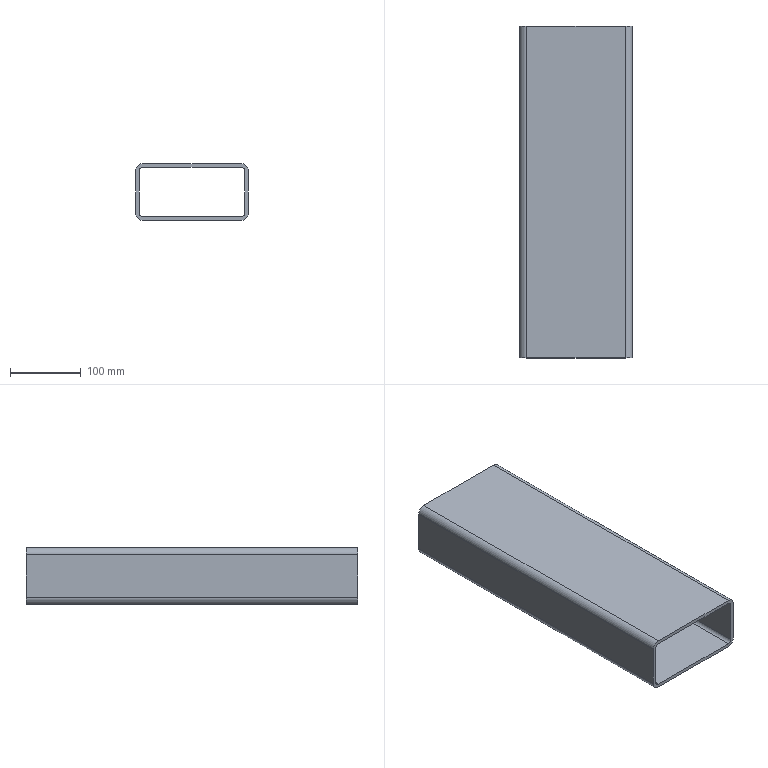Part | SolidWorks | features BaseBody 1 | 1 solid | 26 faces | box 160 x 470 x 80 mm | volume 1049107 mm3 | cylinder 16 | plane 10 | commonest cylinder face diameters 10.2 x8 10 x4 20 x4
STEP:
#1=CARTESIAN_POINT('',(-30.1,174.36,-35.));
#2=VERTEX_POINT('',#1);
#3=CARTESIAN_POINT('',(-19.9,174.36,-35.));
#4=VERTEX_POINT('',#3);
#5=CARTESIAN_POINT('',(-25.,174.36,-35.));
#6=DIRECTION('',(0.,0.,1.));
#7=DIRECTION('',(1.,0.,0.));
#8=AXIS2_PLACEMENT_3D('',#5,#6,#7);
#9=CIRCLE('',#8,5.1);
#10=EDGE_CURVE('',#2,#4,#9,.T.);
#11=ORIENTED_EDGE('',*,*,#10,.T.);
#12=CARTESIAN_POINT('',(-19.9,174.36,-40.));
#13=VERTEX_POINT('',#12);
#14=CARTESIAN_POINT('',(-19.9,174.36,-54.));
#15=DIRECTION('',(0.,0.,-1.));
#16=VECTOR('',#15,1000.);
#17=LINE('',#14,#16);
#18=EDGE_CURVE('',#4,#13,#17,.T.);
#19=ORIENTED_EDGE('',*,*,#18,.T.);
#20=CARTESIAN_POINT('',(-30.1,174.36,-40.));
#21=VERTEX_POINT('',#20);
#22=CARTESIAN_POINT('',(-25.,174.36,-40.));
#23=DIRECTION('',(0.,0.,1.));
#24=DIRECTION('',(1.,0.,0.));
#25=AXIS2_PLACEMENT_3D('',#22,#23,#24);
#26=CIRCLE('',#25,5.1);
#27=EDGE_CURVE('',#21,#13,#26,.T.);
#28=ORIENTED_EDGE('',*,*,#27,.F.);
#29=CARTESIAN_POINT('',(-30.1,174.36,-54.));
#30=DIRECTION('',(0.,0.,-1.));
#31=VECTOR('',#30,1000.);
#32=LINE('',#29,#31);
#33=EDGE_CURVE('',#2,#21,#32,.T.);
#34=ORIENTED_EDGE('',*,*,#33,.F.);
#35=EDGE_LOOP('',(#11,#19,#28,#34));
#36=FACE_OUTER_BOUND('',#35,.T.);
#37=CARTESIAN_POINT('',(-25.,174.36,-54.));
#38=DIRECTION('',(0.,0.,-1.));
#39=DIRECTION('',(-1.,0.,0.));
#40=AXIS2_PLACEMENT_3D('',#37,#38,#39);
#41=CYLINDRICAL_SURFACE('',#40,5.1);
#42=ADVANCED_FACE('',(#36),#41,.F.);
#43=CARTESIAN_POINT('',(29.9,174.36,-35.));
#44=VERTEX_POINT('',#43);
#45=CARTESIAN_POINT('',(40.1,174.36,-35.));
#46=VERTEX_POINT('',#45);
#47=CARTESIAN_POINT('',(35.,174.36,-35.));
#48=DIRECTION('',(0.,0.,1.));
#49=DIRECTION('',(1.,0.,0.));
#50=AXIS2_PLACEMENT_3D('',#47,#48,#49);
#51=CIRCLE('',#50,5.1);
#52=EDGE_CURVE('',#44,#46,#51,.T.);
#53=ORIENTED_EDGE('',*,*,#52,.T.);
#54=CARTESIAN_POINT('',(40.1,174.36,-40.));
#55=VERTEX_POINT('',#54);
#56=CARTESIAN_POINT('',(40.1,174.36,-54.));
#57=DIRECTION('',(0.,0.,-1.));
#58=VECTOR('',#57,1000.);
#59=LINE('',#56,#58);
#60=EDGE_CURVE('',#46,#55,#59,.T.);
#61=ORIENTED_EDGE('',*,*,#60,.T.);
#62=CARTESIAN_POINT('',(29.9,174.36,-40.));
#63=VERTEX_POINT('',#62);
#64=CARTESIAN_POINT('',(35.,174.36,-40.));
#65=DIRECTION('',(0.,0.,1.));
#66=DIRECTION('',(1.,0.,0.));
#67=AXIS2_PLACEMENT_3D('',#64,#65,#66);
#68=CIRCLE('',#67,5.1);
#69=EDGE_CURVE('',#63,#55,#68,.T.);
#70=ORIENTED_EDGE('',*,*,#69,.F.);
#71=CARTESIAN_POINT('',(29.9,174.36,-54.));
#72=DIRECTION('',(0.,0.,-1.));
#73=VECTOR('',#72,1000.);
#74=LINE('',#71,#73);
#75=EDGE_CURVE('',#44,#63,#74,.T.);
#76=ORIENTED_EDGE('',*,*,#75,.F.);
#77=EDGE_LOOP('',(#53,#61,#70,#76));
#78=FACE_OUTER_BOUND('',#77,.T.);
#79=CARTESIAN_POINT('',(35.,174.36,-54.));
#80=DIRECTION('',(0.,0.,-1.));
#81=DIRECTION('',(-1.,0.,0.));
#82=AXIS2_PLACEMENT_3D('',#79,#80,#81);
#83=CYLINDRICAL_SURFACE('',#82,5.1);
#84=ADVANCED_FACE('',(#78),#83,.F.);
#85=CARTESIAN_POINT('',(29.9,54.36,-35.));
#86=VERTEX_POINT('',#85);
#87=CARTESIAN_POINT('',(40.1,54.36,-35.));
#88=VERTEX_POINT('',#87);
#89=CARTESIAN_POINT('',(35.,54.36,-35.));
#90=DIRECTION('',(0.,0.,1.));
#91=DIRECTION('',(1.,0.,0.));
#92=AXIS2_PLACEMENT_3D('',#89,#90,#91);
#93=CIRCLE('',#92,5.1);
#94=EDGE_CURVE('',#86,#88,#93,.T.);
#95=ORIENTED_EDGE('',*,*,#94,.T.);
#96=CARTESIAN_POINT('',(40.1,54.36,-40.));
#97=VERTEX_POINT('',#96);
#98=CARTESIAN_POINT('',(40.1,54.36,-54.));
#99=DIRECTION('',(0.,0.,-1.));
#100=VECTOR('',#99,1000.);
#101=LINE('',#98,#100);
#102=EDGE_CURVE('',#88,#97,#101,.T.);
#103=ORIENTED_EDGE('',*,*,#102,.T.);
#104=CARTESIAN_POINT('',(29.9,54.36,-40.));
#105=VERTEX_POINT('',#104);
#106=CARTESIAN_POINT('',(35.,54.36,-40.));
#107=DIRECTION('',(0.,0.,1.));
#108=DIRECTION('',(1.,0.,0.));
#109=AXIS2_PLACEMENT_3D('',#106,#107,#108);
#110=CIRCLE('',#109,5.1);
#111=EDGE_CURVE('',#105,#97,#110,.T.);
#112=ORIENTED_EDGE('',*,*,#111,.F.);
#113=CARTESIAN_POINT('',(29.9,54.36,-54.));
#114=DIRECTION('',(0.,0.,-1.));
#115=VECTOR('',#114,1000.);
#116=LINE('',#113,#115);
#117=EDGE_CURVE('',#86,#105,#116,.T.);
#118=ORIENTED_EDGE('',*,*,#117,.F.);
#119=EDGE_LOOP('',(#95,#103,#112,#118));
#120=FACE_OUTER_BOUND('',#119,.T.);
#121=CARTESIAN_POINT('',(35.,54.36,-54.));
#122=DIRECTION('',(0.,0.,-1.));
#123=DIRECTION('',(-1.,0.,0.));
#124=AXIS2_PLACEMENT_3D('',#121,#122,#123);
#125=CYLINDRICAL_SURFACE('',#124,5.1);
#126=ADVANCED_FACE('',(#120),#125,.F.);
#127=CARTESIAN_POINT('',(-30.1,54.36,-35.));
#128=VERTEX_POINT('',#127);
#129=CARTESIAN_POINT('',(-19.9,54.36,-35.));
#130=VERTEX_POINT('',#129);
#131=CARTESIAN_POINT('',(-25.,54.36,-35.));
#132=DIRECTION('',(0.,0.,1.));
#133=DIRECTION('',(1.,0.,0.));
#134=AXIS2_PLACEMENT_3D('',#131,#132,#133);
#135=CIRCLE('',#134,5.1);
#136=EDGE_CURVE('',#128,#130,#135,.T.);
#137=ORIENTED_EDGE('',*,*,#136,.T.);
#138=CARTESIAN_POINT('',(-19.9,54.36,-40.));
#139=VERTEX_POINT('',#138);
#140=CARTESIAN_POINT('',(-19.9,54.36,-54.));
#141=DIRECTION('',(0.,0.,-1.));
#142=VECTOR('',#141,1000.);
#143=LINE('',#140,#142);
#144=EDGE_CURVE('',#130,#139,#143,.T.);
#145=ORIENTED_EDGE('',*,*,#144,.T.);
#146=CARTESIAN_POINT('',(-30.1,54.36,-40.));
#147=VERTEX_POINT('',#146);
#148=CARTESIAN_POINT('',(-25.,54.36,-40.));
#149=DIRECTION('',(0.,0.,1.));
#150=DIRECTION('',(1.,0.,0.));
#151=AXIS2_PLACEMENT_3D('',#148,#149,#150);
#152=CIRCLE('',#151,5.1);
#153=EDGE_CURVE('',#147,#139,#152,.T.);
#154=ORIENTED_EDGE('',*,*,#153,.F.);
#155=CARTESIAN_POINT('',(-30.1,54.36,-54.));
#156=DIRECTION('',(0.,0.,-1.));
#157=VECTOR('',#156,1000.);
#158=LINE('',#155,#157);
#159=EDGE_CURVE('',#128,#147,#158,.T.);
#160=ORIENTED_EDGE('',*,*,#159,.F.);
#161=EDGE_LOOP('',(#137,#145,#154,#160));
#162=FACE_OUTER_BOUND('',#161,.T.);
#163=CARTESIAN_POINT('',(-25.,54.36,-54.));
#164=DIRECTION('',(0.,0.,-1.));
#165=DIRECTION('',(-1.,0.,0.));
#166=AXIS2_PLACEMENT_3D('',#163,#164,#165);
#167=CYLINDRICAL_SURFACE('',#166,5.1);
#168=ADVANCED_FACE('',(#162),#167,.F.);
#169=CARTESIAN_POINT('',(-70.,235.,40.));
#170=VERTEX_POINT('',#169);
#171=CARTESIAN_POINT('',(-80.,235.,30.));
#172=VERTEX_POINT('',#171);
#173=CARTESIAN_POINT('',(-70.,235.,30.));
#174=DIRECTION('',(0.,-1.,0.));
#175=DIRECTION('',(1.,0.,0.));
#176=AXIS2_PLACEMENT_3D('',#173,#174,#175);
#177=CIRCLE('',#176,10.);
#178=EDGE_CURVE('',#170,#172,#177,.T.);
#179=ORIENTED_EDGE('',*,*,#178,.T.);
#180=CARTESIAN_POINT('',(-80.,-235.,30.));
#181=VERTEX_POINT('',#180);
#182=CARTESIAN_POINT('',(-80.,-235.,30.));
#183=DIRECTION('',(0.,1.,0.));
#184=VECTOR('',#183,1000.);
#185=LINE('',#182,#184);
#186=EDGE_CURVE('',#181,#172,#185,.T.);
#187=ORIENTED_EDGE('',*,*,#186,.F.);
#188=CARTESIAN_POINT('',(-70.,-235.,40.));
#189=VERTEX_POINT('',#188);
#190=CARTESIAN_POINT('',(-70.,-235.,30.));
#191=DIRECTION('',(0.,-1.,0.));
#192=DIRECTION('',(1.,0.,0.));
#193=AXIS2_PLACEMENT_3D('',#190,#191,#192);
#194=CIRCLE('',#193,10.);
#195=EDGE_CURVE('',#189,#181,#194,.T.);
#196=ORIENTED_EDGE('',*,*,#195,.F.);
#197=CARTESIAN_POINT('',(-70.,-235.,40.));
#198=DIRECTION('',(0.,1.,0.));
#199=VECTOR('',#198,1000.);
#200=LINE('',#197,#199);
#201=EDGE_CURVE('',#189,#170,#200,.T.);
#202=ORIENTED_EDGE('',*,*,#201,.T.);
#203=EDGE_LOOP('',(#179,#187,#196,#202));
#204=FACE_OUTER_BOUND('',#203,.T.);
#205=CARTESIAN_POINT('',(-70.,-235.,30.));
#206=DIRECTION('',(0.,1.,0.));
#207=DIRECTION('',(-1.,0.,0.));
#208=AXIS2_PLACEMENT_3D('',#205,#206,#207);
#209=CYLINDRICAL_SURFACE('',#208,10.);
#210=ADVANCED_FACE('',(#204),#209,.T.);
#211=CARTESIAN_POINT('',(-80.,235.,-30.));
#212=VERTEX_POINT('',#211);
#213=CARTESIAN_POINT('',(-80.,235.,30.));
#214=DIRECTION('',(0.,0.,-1.));
#215=VECTOR('',#214,1000.);
#216=LINE('',#213,#215);
#217=EDGE_CURVE('',#172,#212,#216,.T.);
#218=ORIENTED_EDGE('',*,*,#217,.T.);
#219=CARTESIAN_POINT('',(-80.,-235.,-30.));
#220=VERTEX_POINT('',#219);
#221=CARTESIAN_POINT('',(-80.,-235.,-30.));
#222=DIRECTION('',(0.,1.,0.));
#223=VECTOR('',#222,1000.);
#224=LINE('',#221,#223);
#225=EDGE_CURVE('',#220,#212,#224,.T.);
#226=ORIENTED_EDGE('',*,*,#225,.F.);
#227=CARTESIAN_POINT('',(-80.,-235.,30.));
#228=DIRECTION('',(0.,0.,-1.));
#229=VECTOR('',#228,1000.);
#230=LINE('',#227,#229);
#231=EDGE_CURVE('',#181,#220,#230,.T.);
#232=ORIENTED_EDGE('',*,*,#231,.F.);
#233=ORIENTED_EDGE('',*,*,#186,.T.);
#234=EDGE_LOOP('',(#218,#226,#232,#233));
#235=FACE_OUTER_BOUND('',#234,.T.);
#236=CARTESIAN_POINT('',(-80.,-235.,30.));
#237=DIRECTION('',(1.,0.,0.));
#238=DIRECTION('',(0.,0.,-1.));
#239=AXIS2_PLACEMENT_3D('',#236,#237,#238);
#240=PLANE('',#239);
#241=ADVANCED_FACE('',(#235),#240,.F.);
#242=CARTESIAN_POINT('',(-70.,235.,-40.));
#243=VERTEX_POINT('',#242);
#244=CARTESIAN_POINT('',(-70.,235.,-30.));
#245=DIRECTION('',(0.,-1.,0.));
#246=DIRECTION('',(1.,0.,0.));
#247=AXIS2_PLACEMENT_3D('',#244,#245,#246);
#248=CIRCLE('',#247,10.);
#249=EDGE_CURVE('',#212,#243,#248,.T.);
#250=ORIENTED_EDGE('',*,*,#249,.T.);
#251=CARTESIAN_POINT('',(-70.,-235.,-40.));
#252=VERTEX_POINT('',#251);
#253=CARTESIAN_POINT('',(-70.,-235.,-40.));
#254=DIRECTION('',(0.,1.,0.));
#255=VECTOR('',#254,1000.);
#256=LINE('',#253,#255);
#257=EDGE_CURVE('',#252,#243,#256,.T.);
#258=ORIENTED_EDGE('',*,*,#257,.F.);
#259=CARTESIAN_POINT('',(-70.,-235.,-30.));
#260=DIRECTION('',(0.,-1.,0.));
#261=DIRECTION('',(1.,0.,0.));
#262=AXIS2_PLACEMENT_3D('',#259,#260,#261);
#263=CIRCLE('',#262,10.);
#264=EDGE_CURVE('',#220,#252,#263,.T.);
#265=ORIENTED_EDGE('',*,*,#264,.F.);
#266=ORIENTED_EDGE('',*,*,#225,.T.);
#267=EDGE_LOOP('',(#250,#258,#265,#266));
#268=FACE_OUTER_BOUND('',#267,.T.);
#269=CARTESIAN_POINT('',(-70.,-235.,-30.));
#270=DIRECTION('',(0.,1.,0.));
#271=DIRECTION('',(-1.,0.,0.));
#272=AXIS2_PLACEMENT_3D('',#269,#270,#271);
#273=CYLINDRICAL_SURFACE('',#272,10.);
#274=ADVANCED_FACE('',(#268),#273,.T.);
#275=ORIENTED_EDGE('',*,*,#27,.T.);
#276=CARTESIAN_POINT('',(-25.,174.36,-40.));
#277=DIRECTION('',(0.,0.,1.));
#278=DIRECTION('',(1.,0.,0.));
#279=AXIS2_PLACEMENT_3D('',#276,#277,#278);
#280=CIRCLE('',#279,5.1);
#281=EDGE_CURVE('',#13,#21,#280,.T.);
#282=ORIENTED_EDGE('',*,*,#281,.T.);
#283=EDGE_LOOP('',(#275,#282));
#284=FACE_BOUND('',#283,.T.);
#285=ORIENTED_EDGE('',*,*,#69,.T.);
#286=CARTESIAN_POINT('',(35.,174.36,-40.));
#287=DIRECTION('',(0.,0.,1.));
#288=DIRECTION('',(1.,0.,0.));
#289=AXIS2_PLACEMENT_3D('',#286,#287,#288);
#290=CIRCLE('',#289,5.1);
#291=EDGE_CURVE('',#55,#63,#290,.T.);
#292=ORIENTED_EDGE('',*,*,#291,.T.);
#293=EDGE_LOOP('',(#285,#292));
#294=FACE_BOUND('',#293,.T.);
#295=ORIENTED_EDGE('',*,*,#111,.T.);
#296=CARTESIAN_POINT('',(35.,54.36,-40.));
#297=DIRECTION('',(0.,0.,1.));
#298=DIRECTION('',(1.,0.,0.));
#299=AXIS2_PLACEMENT_3D('',#296,#297,#298);
#300=CIRCLE('',#299,5.1);
#301=EDGE_CURVE('',#97,#105,#300,.T.);
#302=ORIENTED_EDGE('',*,*,#301,.T.);
#303=EDGE_LOOP('',(#295,#302));
#304=FACE_BOUND('',#303,.T.);
#305=ORIENTED_EDGE('',*,*,#153,.T.);
#306=CARTESIAN_POINT('',(-25.,54.36,-40.));
#307=DIRECTION('',(0.,0.,1.));
#308=DIRECTION('',(1.,0.,0.));
#309=AXIS2_PLACEMENT_3D('',#306,#307,#308);
#310=CIRCLE('',#309,5.1);
#311=EDGE_CURVE('',#139,#147,#310,.T.);
#312=ORIENTED_EDGE('',*,*,#311,.T.);
#313=EDGE_LOOP('',(#305,#312));
#314=FACE_BOUND('',#313,.T.);
#315=CARTESIAN_POINT('',(70.,235.,-40.));
#316=VERTEX_POINT('',#315);
#317=CARTESIAN_POINT('',(70.,235.,-40.));
#318=DIRECTION('',(1.,0.,0.));
#319=VECTOR('',#318,1000.);
#320=LINE('',#317,#319);
#321=EDGE_CURVE('',#243,#316,#320,.T.);
#322=ORIENTED_EDGE('',*,*,#321,.T.);
#323=CARTESIAN_POINT('',(70.,-235.,-40.));
#324=VERTEX_POINT('',#323);
#325=CARTESIAN_POINT('',(70.,-235.,-40.));
#326=DIRECTION('',(0.,1.,0.));
#327=VECTOR('',#326,1000.);
#328=LINE('',#325,#327);
#329=EDGE_CURVE('',#324,#316,#328,.T.);
#330=ORIENTED_EDGE('',*,*,#329,.F.);
#331=CARTESIAN_POINT('',(70.,-235.,-40.));
#332=DIRECTION('',(1.,0.,0.));
#333=VECTOR('',#332,1000.);
#334=LINE('',#331,#333);
#335=EDGE_CURVE('',#252,#324,#334,.T.);
#336=ORIENTED_EDGE('',*,*,#335,.F.);
#337=ORIENTED_EDGE('',*,*,#257,.T.);
#338=EDGE_LOOP('',(#322,#330,#336,#337));
#339=FACE_OUTER_BOUND('',#338,.T.);
#340=CARTESIAN_POINT('',(70.,-235.,-40.));
#341=DIRECTION('',(0.,0.,1.));
#342=DIRECTION('',(1.,0.,0.));
#343=AXIS2_PLACEMENT_3D('',#340,#341,#342);
#344=PLANE('',#343);
#345=ADVANCED_FACE('',(#284,#294,#304,#314,#339),#344,.F.);
#346=CARTESIAN_POINT('',(80.,235.,-30.));
#347=VERTEX_POINT('',#346);
#348=CARTESIAN_POINT('',(70.,235.,-30.));
#349=DIRECTION('',(0.,-1.,0.));
#350=DIRECTION('',(1.,0.,0.));
#351=AXIS2_PLACEMENT_3D('',#348,#349,#350);
#352=CIRCLE('',#351,10.);
#353=EDGE_CURVE('',#316,#347,#352,.T.);
#354=ORIENTED_EDGE('',*,*,#353,.T.);
#355=CARTESIAN_POINT('',(80.,-235.,-30.));
#356=VERTEX_POINT('',#355);
#357=CARTESIAN_POINT('',(80.,-235.,-30.));
#358=DIRECTION('',(0.,1.,0.));
#359=VECTOR('',#358,1000.);
#360=LINE('',#357,#359);
#361=EDGE_CURVE('',#356,#347,#360,.T.);
#362=ORIENTED_EDGE('',*,*,#361,.F.);
#363=CARTESIAN_POINT('',(70.,-235.,-30.));
#364=DIRECTION('',(0.,-1.,0.));
#365=DIRECTION('',(1.,0.,0.));
#366=AXIS2_PLACEMENT_3D('',#363,#364,#365);
#367=CIRCLE('',#366,10.);
#368=EDGE_CURVE('',#324,#356,#367,.T.);
#369=ORIENTED_EDGE('',*,*,#368,.F.);
#370=ORIENTED_EDGE('',*,*,#329,.T.);
#371=EDGE_LOOP('',(#354,#362,#369,#370));
#372=FACE_OUTER_BOUND('',#371,.T.);
#373=CARTESIAN_POINT('',(70.,-235.,-30.));
#374=DIRECTION('',(0.,1.,0.));
#375=DIRECTION('',(-1.,0.,0.));
#376=AXIS2_PLACEMENT_3D('',#373,#374,#375);
#377=CYLINDRICAL_SURFACE('',#376,10.);
#378=ADVANCED_FACE('',(#372),#377,.T.);
#379=CARTESIAN_POINT('',(80.,235.,30.));
#380=VERTEX_POINT('',#379);
#381=CARTESIAN_POINT('',(80.,235.,-30.));
#382=DIRECTION('',(0.,0.,1.));
#383=VECTOR('',#382,1000.);
#384=LINE('',#381,#383);
#385=EDGE_CURVE('',#347,#380,#384,.T.);
#386=ORIENTED_EDGE('',*,*,#385,.T.);
#387=CARTESIAN_POINT('',(80.,-235.,30.));
#388=VERTEX_POINT('',#387);
#389=CARTESIAN_POINT('',(80.,-235.,30.));
#390=DIRECTION('',(0.,1.,0.));
#391=VECTOR('',#390,1000.);
#392=LINE('',#389,#391);
#393=EDGE_CURVE('',#388,#380,#392,.T.);
#394=ORIENTED_EDGE('',*,*,#393,.F.);
#395=CARTESIAN_POINT('',(80.,-235.,-30.));
#396=DIRECTION('',(0.,0.,1.));
#397=VECTOR('',#396,1000.);
#398=LINE('',#395,#397);
#399=EDGE_CURVE('',#356,#388,#398,.T.);
#400=ORIENTED_EDGE('',*,*,#399,.F.);
#401=ORIENTED_EDGE('',*,*,#361,.T.);
#402=EDGE_LOOP('',(#386,#394,#400,#401));
#403=FACE_OUTER_BOUND('',#402,.T.);
#404=CARTESIAN_POINT('',(80.,-235.,-30.));
#405=DIRECTION('',(-1.,0.,0.));
#406=DIRECTION('',(0.,0.,1.));
#407=AXIS2_PLACEMENT_3D('',#404,#405,#406);
#408=PLANE('',#407);
#409=ADVANCED_FACE('',(#403),#408,.F.);
#410=CARTESIAN_POINT('',(70.,235.,40.));
#411=VERTEX_POINT('',#410);
#412=CARTESIAN_POINT('',(70.,235.,30.));
#413=DIRECTION('',(0.,-1.,0.));
#414=DIRECTION('',(1.,0.,0.));
#415=AXIS2_PLACEMENT_3D('',#412,#413,#414);
#416=CIRCLE('',#415,10.);
#417=EDGE_CURVE('',#380,#411,#416,.T.);
#418=ORIENTED_EDGE('',*,*,#417,.T.);
#419=CARTESIAN_POINT('',(70.,-235.,40.));
#420=VERTEX_POINT('',#419);
#421=CARTESIAN_POINT('',(70.,-235.,40.));
#422=DIRECTION('',(0.,1.,0.));
#423=VECTOR('',#422,1000.);
#424=LINE('',#421,#423);
#425=EDGE_CURVE('',#420,#411,#424,.T.);
#426=ORIENTED_EDGE('',*,*,#425,.F.);
#427=CARTESIAN_POINT('',(70.,-235.,30.));
#428=DIRECTION('',(0.,-1.,0.));
#429=DIRECTION('',(1.,0.,0.));
#430=AXIS2_PLACEMENT_3D('',#427,#428,#429);
#431=CIRCLE('',#430,10.);
#432=EDGE_CURVE('',#388,#420,#431,.T.);
#433=ORIENTED_EDGE('',*,*,#432,.F.);
#434=ORIENTED_EDGE('',*,*,#393,.T.);
#435=EDGE_LOOP('',(#418,#426,#433,#434));
#436=FACE_OUTER_BOUND('',#435,.T.);
#437=CARTESIAN_POINT('',(70.,-235.,30.));
#438=DIRECTION('',(0.,1.,0.));
#439=DIRECTION('',(-1.,0.,0.));
#440=AXIS2_PLACEMENT_3D('',#437,#438,#439);
#441=CYLINDRICAL_SURFACE('',#440,10.);
#442=ADVANCED_FACE('',(#436),#441,.T.);
#443=CARTESIAN_POINT('',(-75.,235.,-30.));
#444=VERTEX_POINT('',#443);
#445=CARTESIAN_POINT('',(-70.,235.,-35.));
#446=VERTEX_POINT('',#445);
#447=CARTESIAN_POINT('',(-70.,235.,-30.));
#448=DIRECTION('',(0.,-1.,0.));
#449=DIRECTION('',(1.,0.,0.));
#450=AXIS2_PLACEMENT_3D('',#447,#448,#449);
#451=CIRCLE('',#450,5.);
#452=EDGE_CURVE('',#444,#446,#451,.T.);
#453=ORIENTED_EDGE('',*,*,#452,.F.);
#454=CARTESIAN_POINT('',(-75.,-235.,-30.));
#455=VERTEX_POINT('',#454);
#456=CARTESIAN_POINT('',(-75.,-235.,-30.));
#457=DIRECTION('',(0.,1.,0.));
#458=VECTOR('',#457,1000.);
#459=LINE('',#456,#458);
#460=EDGE_CURVE('',#455,#444,#459,.T.);
#461=ORIENTED_EDGE('',*,*,#460,.F.);
#462=CARTESIAN_POINT('',(-70.,-235.,-35.));
#463=VERTEX_POINT('',#462);
#464=CARTESIAN_POINT('',(-70.,-235.,-30.));
#465=DIRECTION('',(0.,-1.,0.));
#466=DIRECTION('',(1.,0.,0.));
#467=AXIS2_PLACEMENT_3D('',#464,#465,#466);
#468=CIRCLE('',#467,5.);
#469=EDGE_CURVE('',#455,#463,#468,.T.);
#470=ORIENTED_EDGE('',*,*,#469,.T.);
#471=CARTESIAN_POINT('',(-70.,-235.,-35.));
#472=DIRECTION('',(0.,1.,0.));
#473=VECTOR('',#472,1000.);
#474=LINE('',#471,#473);
#475=EDGE_CURVE('',#463,#446,#474,.T.);
#476=ORIENTED_EDGE('',*,*,#475,.T.);
#477=EDGE_LOOP('',(#453,#461,#470,#476));
#478=FACE_OUTER_BOUND('',#477,.T.);
#479=CARTESIAN_POINT('',(-70.,-235.,-30.));
#480=DIRECTION('',(0.,1.,0.));
#481=DIRECTION('',(-1.,0.,0.));
#482=AXIS2_PLACEMENT_3D('',#479,#480,#481);
#483=CYLINDRICAL_SURFACE('',#482,5.);
#484=ADVANCED_FACE('',(#478),#483,.F.);
#485=CARTESIAN_POINT('',(-75.,235.,30.));
#486=VERTEX_POINT('',#485);
#487=CARTESIAN_POINT('',(-75.,235.,30.));
#488=DIRECTION('',(0.,0.,-1.));
#489=VECTOR('',#488,1000.);
#490=LINE('',#487,#489);
#491=EDGE_CURVE('',#486,#444,#490,.T.);
#492=ORIENTED_EDGE('',*,*,#491,.F.);
#493=CARTESIAN_POINT('',(-75.,-235.,30.));
#494=VERTEX_POINT('',#493);
#495=CARTESIAN_POINT('',(-75.,-235.,30.));
#496=DIRECTION('',(0.,1.,0.));
#497=VECTOR('',#496,1000.);
#498=LINE('',#495,#497);
#499=EDGE_CURVE('',#494,#486,#498,.T.);
#500=ORIENTED_EDGE('',*,*,#499,.F.);
#501=CARTESIAN_POINT('',(-75.,-235.,30.));
#502=DIRECTION('',(0.,0.,-1.));
#503=VECTOR('',#502,1000.);
#504=LINE('',#501,#503);
#505=EDGE_CURVE('',#494,#455,#504,.T.);
#506=ORIENTED_EDGE('',*,*,#505,.T.);
#507=ORIENTED_EDGE('',*,*,#460,.T.);
#508=EDGE_LOOP('',(#492,#500,#506,#507));
#509=FACE_OUTER_BOUND('',#508,.T.);
#510=CARTESIAN_POINT('',(-75.,-235.,30.));
#511=DIRECTION('',(1.,0.,0.));
#512=DIRECTION('',(0.,0.,-1.));
#513=AXIS2_PLACEMENT_3D('',#510,#511,#512);
#514=PLANE('',#513);
#515=ADVANCED_FACE('',(#509),#514,.T.);
#516=CARTESIAN_POINT('',(-70.,235.,35.));
#517=VERTEX_POINT('',#516);
#518=CARTESIAN_POINT('',(-70.,235.,30.));
#519=DIRECTION('',(0.,-1.,0.));
#520=DIRECTION('',(1.,0.,0.));
#521=AXIS2_PLACEMENT_3D('',#518,#519,#520);
#522=CIRCLE('',#521,5.);
#523=EDGE_CURVE('',#517,#486,#522,.T.);
#524=ORIENTED_EDGE('',*,*,#523,.F.);
#525=CARTESIAN_POINT('',(-70.,-235.,35.));
#526=VERTEX_POINT('',#525);
#527=CARTESIAN_POINT('',(-70.,-235.,35.));
#528=DIRECTION('',(0.,1.,0.));
#529=VECTOR('',#528,1000.);
#530=LINE('',#527,#529);
#531=EDGE_CURVE('',#526,#517,#530,.T.);
#532=ORIENTED_EDGE('',*,*,#531,.F.);
#533=CARTESIAN_POINT('',(-70.,-235.,30.));
#534=DIRECTION('',(0.,-1.,0.));
#535=DIRECTION('',(1.,0.,0.));
#536=AXIS2_PLACEMENT_3D('',#533,#534,#535);
#537=CIRCLE('',#536,5.);
#538=EDGE_CURVE('',#526,#494,#537,.T.);
#539=ORIENTED_EDGE('',*,*,#538,.T.);
#540=ORIENTED_EDGE('',*,*,#499,.T.);
#541=EDGE_LOOP('',(#524,#532,#539,#540));
#542=FACE_OUTER_BOUND('',#541,.T.);
#543=CARTESIAN_POINT('',(-70.,-235.,30.));
#544=DIRECTION('',(0.,1.,0.));
#545=DIRECTION('',(-1.,0.,0.));
#546=AXIS2_PLACEMENT_3D('',#543,#544,#545);
#547=CYLINDRICAL_SURFACE('',#546,5.);
#548=ADVANCED_FACE('',(#542),#547,.F.);
#549=CARTESIAN_POINT('',(70.,235.,35.));
#550=VERTEX_POINT('',#549);
#551=CARTESIAN_POINT('',(-70.,235.,35.));
#552=DIRECTION('',(-1.,0.,0.));
#553=VECTOR('',#552,1000.);
#554=LINE('',#551,#553);
#555=EDGE_CURVE('',#550,#517,#554,.T.);
#556=ORIENTED_EDGE('',*,*,#555,.F.);
#557=CARTESIAN_POINT('',(70.,-235.,35.));
#558=VERTEX_POINT('',#557);
#559=CARTESIAN_POINT('',(70.,-235.,35.));
#560=DIRECTION('',(0.,1.,0.));
#561=VECTOR('',#560,1000.);
#562=LINE('',#559,#561);
#563=EDGE_CURVE('',#558,#550,#562,.T.);
#564=ORIENTED_EDGE('',*,*,#563,.F.);
#565=CARTESIAN_POINT('',(-70.,-235.,35.));
#566=DIRECTION('',(-1.,0.,0.));
#567=VECTOR('',#566,1000.);
#568=LINE('',#565,#567);
#569=EDGE_CURVE('',#558,#526,#568,.T.);
#570=ORIENTED_EDGE('',*,*,#569,.T.);
#571=ORIENTED_EDGE('',*,*,#531,.T.);
#572=EDGE_LOOP('',(#556,#564,#570,#571));
#573=FACE_OUTER_BOUND('',#572,.T.);
#574=CARTESIAN_POINT('',(-70.,-235.,35.));
#575=DIRECTION('',(0.,0.,-1.));
#576=DIRECTION('',(-1.,0.,0.));
#577=AXIS2_PLACEMENT_3D('',#574,#575,#576);
#578=PLANE('',#577);
#579=ADVANCED_FACE('',(#573),#578,.T.);
#580=CARTESIAN_POINT('',(75.,235.,30.));
#581=VERTEX_POINT('',#580);
#582=CARTESIAN_POINT('',(70.,235.,30.));
#583=DIRECTION('',(0.,-1.,0.));
#584=DIRECTION('',(1.,0.,0.));
#585=AXIS2_PLACEMENT_3D('',#582,#583,#584);
#586=CIRCLE('',#585,5.);
#587=EDGE_CURVE('',#581,#550,#586,.T.);
#588=ORIENTED_EDGE('',*,*,#587,.F.);
#589=CARTESIAN_POINT('',(75.,-235.,30.));
#590=VERTEX_POINT('',#589);
#591=CARTESIAN_POINT('',(75.,-235.,30.));
#592=DIRECTION('',(0.,1.,0.));
#593=VECTOR('',#592,1000.);
#594=LINE('',#591,#593);
#595=EDGE_CURVE('',#590,#581,#594,.T.);
#596=ORIENTED_EDGE('',*,*,#595,.F.);
#597=CARTESIAN_POINT('',(70.,-235.,30.));
#598=DIRECTION('',(0.,-1.,0.));
#599=DIRECTION('',(1.,0.,0.));
#600=AXIS2_PLACEMENT_3D('',#597,#598,#599);
#601=CIRCLE('',#600,5.);
#602=EDGE_CURVE('',#590,#558,#601,.T.);
#603=ORIENTED_EDGE('',*,*,#602,.T.);
#604=ORIENTED_EDGE('',*,*,#563,.T.);
#605=EDGE_LOOP('',(#588,#596,#603,#604));
#606=FACE_OUTER_BOUND('',#605,.T.);
#607=CARTESIAN_POINT('',(70.,-235.,30.));
#608=DIRECTION('',(0.,1.,0.));
#609=DIRECTION('',(-1.,0.,0.));
#610=AXIS2_PLACEMENT_3D('',#607,#608,#609);
#611=CYLINDRICAL_SURFACE('',#610,5.);
#612=ADVANCED_FACE('',(#606),#611,.F.);
#613=CARTESIAN_POINT('',(75.,235.,-30.));
#614=VERTEX_POINT('',#613);
#615=CARTESIAN_POINT('',(75.,235.,-30.));
#616=DIRECTION('',(0.,0.,1.));
#617=VECTOR('',#616,1000.);
#618=LINE('',#615,#617);
#619=EDGE_CURVE('',#614,#581,#618,.T.);
#620=ORIENTED_EDGE('',*,*,#619,.F.);
#621=CARTESIAN_POINT('',(75.,-235.,-30.));
#622=VERTEX_POINT('',#621);
#623=CARTESIAN_POINT('',(75.,-235.,-30.));
#624=DIRECTION('',(0.,1.,0.));
#625=VECTOR('',#624,1000.);
#626=LINE('',#623,#625);
#627=EDGE_CURVE('',#622,#614,#626,.T.);
#628=ORIENTED_EDGE('',*,*,#627,.F.);
#629=CARTESIAN_POINT('',(75.,-235.,-30.));
#630=DIRECTION('',(0.,0.,1.));
#631=VECTOR('',#630,1000.);
#632=LINE('',#629,#631);
#633=EDGE_CURVE('',#622,#590,#632,.T.);
#634=ORIENTED_EDGE('',*,*,#633,.T.);
#635=ORIENTED_EDGE('',*,*,#595,.T.);
#636=EDGE_LOOP('',(#620,#628,#634,#635));
#637=FACE_OUTER_BOUND('',#636,.T.);
#638=CARTESIAN_POINT('',(75.,-235.,-30.));
#639=DIRECTION('',(-1.,0.,0.));
#640=DIRECTION('',(0.,0.,1.));
#641=AXIS2_PLACEMENT_3D('',#638,#639,#640);
#642=PLANE('',#641);
#643=ADVANCED_FACE('',(#637),#642,.T.);
#644=CARTESIAN_POINT('',(70.,235.,-35.));
#645=VERTEX_POINT('',#644);
#646=CARTESIAN_POINT('',(70.,235.,-30.));
#647=DIRECTION('',(0.,-1.,0.));
#648=DIRECTION('',(1.,0.,0.));
#649=AXIS2_PLACEMENT_3D('',#646,#647,#648);
#650=CIRCLE('',#649,5.);
#651=EDGE_CURVE('',#645,#614,#650,.T.);
#652=ORIENTED_EDGE('',*,*,#651,.F.);
#653=CARTESIAN_POINT('',(70.,-235.,-35.));
#654=VERTEX_POINT('',#653);
#655=CARTESIAN_POINT('',(70.,-235.,-35.));
#656=DIRECTION('',(0.,1.,0.));
#657=VECTOR('',#656,1000.);
#658=LINE('',#655,#657);
#659=EDGE_CURVE('',#654,#645,#658,.T.);
#660=ORIENTED_EDGE('',*,*,#659,.F.);
#661=CARTESIAN_POINT('',(70.,-235.,-30.));
#662=DIRECTION('',(0.,-1.,0.));
#663=DIRECTION('',(1.,0.,0.));
#664=AXIS2_PLACEMENT_3D('',#661,#662,#663);
#665=CIRCLE('',#664,5.);
#666=EDGE_CURVE('',#654,#622,#665,.T.);
#667=ORIENTED_EDGE('',*,*,#666,.T.);
#668=ORIENTED_EDGE('',*,*,#627,.T.);
#669=EDGE_LOOP('',(#652,#660,#667,#668));
#670=FACE_OUTER_BOUND('',#669,.T.);
#671=CARTESIAN_POINT('',(70.,-235.,-30.));
#672=DIRECTION('',(0.,1.,0.));
#673=DIRECTION('',(-1.,0.,0.));
#674=AXIS2_PLACEMENT_3D('',#671,#672,#673);
#675=CYLINDRICAL_SURFACE('',#674,5.);
#676=ADVANCED_FACE('',(#670),#675,.F.);
#677=ORIENTED_EDGE('',*,*,#10,.F.);
#678=CARTESIAN_POINT('',(-25.,174.36,-35.));
#679=DIRECTION('',(0.,0.,1.));
#680=DIRECTION('',(1.,0.,0.));
#681=AXIS2_PLACEMENT_3D('',#678,#679,#680);
#682=CIRCLE('',#681,5.1);
#683=EDGE_CURVE('',#4,#2,#682,.T.);
#684=ORIENTED_EDGE('',*,*,#683,.F.);
#685=EDGE_LOOP('',(#677,#684));
#686=FACE_BOUND('',#685,.T.);
#687=ORIENTED_EDGE('',*,*,#52,.F.);
#688=CARTESIAN_POINT('',(35.,174.36,-35.));
#689=DIRECTION('',(0.,0.,1.));
#690=DIRECTION('',(1.,0.,0.));
#691=AXIS2_PLACEMENT_3D('',#688,#689,#690);
#692=CIRCLE('',#691,5.1);
#693=EDGE_CURVE('',#46,#44,#692,.T.);
#694=ORIENTED_EDGE('',*,*,#693,.F.);
#695=EDGE_LOOP('',(#687,#694));
#696=FACE_BOUND('',#695,.T.);
#697=ORIENTED_EDGE('',*,*,#94,.F.);
#698=CARTESIAN_POINT('',(35.,54.36,-35.));
#699=DIRECTION('',(0.,0.,1.));
#700=DIRECTION('',(1.,0.,0.));
#701=AXIS2_PLACEMENT_3D('',#698,#699,#700);
#702=CIRCLE('',#701,5.1);
#703=EDGE_CURVE('',#88,#86,#702,.T.);
#704=ORIENTED_EDGE('',*,*,#703,.F.);
#705=EDGE_LOOP('',(#697,#704));
#706=FACE_BOUND('',#705,.T.);
#707=ORIENTED_EDGE('',*,*,#136,.F.);
#708=CARTESIAN_POINT('',(-25.,54.36,-35.));
#709=DIRECTION('',(0.,0.,1.));
#710=DIRECTION('',(1.,0.,0.));
#711=AXIS2_PLACEMENT_3D('',#708,#709,#710);
#712=CIRCLE('',#711,5.1);
#713=EDGE_CURVE('',#130,#128,#712,.T.);
#714=ORIENTED_EDGE('',*,*,#713,.F.);
#715=EDGE_LOOP('',(#707,#714));
#716=FACE_BOUND('',#715,.T.);
#717=CARTESIAN_POINT('',(70.,235.,-35.));
#718=DIRECTION('',(1.,0.,0.));
#719=VECTOR('',#718,1000.);
#720=LINE('',#717,#719);
#721=EDGE_CURVE('',#446,#645,#720,.T.);
#722=ORIENTED_EDGE('',*,*,#721,.F.);
#723=ORIENTED_EDGE('',*,*,#475,.F.);
#724=CARTESIAN_POINT('',(70.,-235.,-35.));
#725=DIRECTION('',(1.,0.,0.));
#726=VECTOR('',#725,1000.);
#727=LINE('',#724,#726);
#728=EDGE_CURVE('',#463,#654,#727,.T.);
#729=ORIENTED_EDGE('',*,*,#728,.T.);
#730=ORIENTED_EDGE('',*,*,#659,.T.);
#731=EDGE_LOOP('',(#722,#723,#729,#730));
#732=FACE_OUTER_BOUND('',#731,.T.);
#733=CARTESIAN_POINT('',(70.,-235.,-35.));
#734=DIRECTION('',(0.,0.,1.));
#735=DIRECTION('',(1.,0.,0.));
#736=AXIS2_PLACEMENT_3D('',#733,#734,#735);
#737=PLANE('',#736);
#738=ADVANCED_FACE('',(#686,#696,#706,#716,#732),#737,.T.);
#739=CARTESIAN_POINT('',(-70.,235.,40.));
#740=DIRECTION('',(-1.,0.,0.));
#741=VECTOR('',#740,1000.);
#742=LINE('',#739,#741);
#743=EDGE_CURVE('',#411,#170,#742,.T.);
#744=ORIENTED_EDGE('',*,*,#743,.T.);
#745=ORIENTED_EDGE('',*,*,#201,.F.);
#746=CARTESIAN_POINT('',(-70.,-235.,40.));
#747=DIRECTION('',(-1.,0.,0.));
#748=VECTOR('',#747,1000.);
#749=LINE('',#746,#748);
#750=EDGE_CURVE('',#420,#189,#749,.T.);
#751=ORIENTED_EDGE('',*,*,#750,.F.);
#752=ORIENTED_EDGE('',*,*,#425,.T.);
#753=EDGE_LOOP('',(#744,#745,#751,#752));
#754=FACE_OUTER_BOUND('',#753,.T.);
#755=CARTESIAN_POINT('',(-70.,-235.,40.));
#756=DIRECTION('',(0.,0.,-1.));
#757=DIRECTION('',(-1.,0.,0.));
#758=AXIS2_PLACEMENT_3D('',#755,#756,#757);
#759=PLANE('',#758);
#760=ADVANCED_FACE('',(#754),#759,.F.);
#761=ORIENTED_EDGE('',*,*,#469,.F.);
#762=ORIENTED_EDGE('',*,*,#505,.F.);
#763=ORIENTED_EDGE('',*,*,#538,.F.);
#764=ORIENTED_EDGE('',*,*,#569,.F.);
#765=ORIENTED_EDGE('',*,*,#602,.F.);
#766=ORIENTED_EDGE('',*,*,#633,.F.);
#767=ORIENTED_EDGE('',*,*,#666,.F.);
#768=ORIENTED_EDGE('',*,*,#728,.F.);
#769=EDGE_LOOP('',(#761,#762,#763,#764,#765,#766,#767,#768));
#770=FACE_BOUND('',#769,.T.);
#771=ORIENTED_EDGE('',*,*,#195,.T.);
#772=ORIENTED_EDGE('',*,*,#231,.T.);
#773=ORIENTED_EDGE('',*,*,#264,.T.);
#774=ORIENTED_EDGE('',*,*,#335,.T.);
#775=ORIENTED_EDGE('',*,*,#368,.T.);
#776=ORIENTED_EDGE('',*,*,#399,.T.);
#777=ORIENTED_EDGE('',*,*,#432,.T.);
#778=ORIENTED_EDGE('',*,*,#750,.T.);
#779=EDGE_LOOP('',(#771,#772,#773,#774,#775,#776,#777,#778));
#780=FACE_OUTER_BOUND('',#779,.T.);
#781=CARTESIAN_POINT('',(-70.,-235.,30.));
#782=DIRECTION('',(0.,-1.,0.));
#783=DIRECTION('',(1.,0.,0.));
#784=AXIS2_PLACEMENT_3D('',#781,#782,#783);
#785=PLANE('',#784);
#786=ADVANCED_FACE('',(#770,#780),#785,.T.);
#787=ORIENTED_EDGE('',*,*,#452,.T.);
#788=ORIENTED_EDGE('',*,*,#721,.T.);
#789=ORIENTED_EDGE('',*,*,#651,.T.);
#790=ORIENTED_EDGE('',*,*,#619,.T.);
#791=ORIENTED_EDGE('',*,*,#587,.T.);
#792=ORIENTED_EDGE('',*,*,#555,.T.);
#793=ORIENTED_EDGE('',*,*,#523,.T.);
#794=ORIENTED_EDGE('',*,*,#491,.T.);
#795=EDGE_LOOP('',(#787,#788,#789,#790,#791,#792,#793,#794));
#796=FACE_BOUND('',#795,.T.);
#797=ORIENTED_EDGE('',*,*,#178,.F.);
#798=ORIENTED_EDGE('',*,*,#743,.F.);
#799=ORIENTED_EDGE('',*,*,#417,.F.);
#800=ORIENTED_EDGE('',*,*,#385,.F.);
#801=ORIENTED_EDGE('',*,*,#353,.F.);
#802=ORIENTED_EDGE('',*,*,#321,.F.);
#803=ORIENTED_EDGE('',*,*,#249,.F.);
#804=ORIENTED_EDGE('',*,*,#217,.F.);
#805=EDGE_LOOP('',(#797,#798,#799,#800,#801,#802,#803,#804));
#806=FACE_OUTER_BOUND('',#805,.T.);
#807=CARTESIAN_POINT('',(-70.,235.,30.));
#808=DIRECTION('',(0.,-1.,0.));
#809=DIRECTION('',(1.,0.,0.));
#810=AXIS2_PLACEMENT_3D('',#807,#808,#809);
#811=PLANE('',#810);
#812=ADVANCED_FACE('',(#796,#806),#811,.F.);
#813=ORIENTED_EDGE('',*,*,#144,.F.);
#814=ORIENTED_EDGE('',*,*,#713,.T.);
#815=ORIENTED_EDGE('',*,*,#159,.T.);
#816=ORIENTED_EDGE('',*,*,#311,.F.);
#817=EDGE_LOOP('',(#813,#814,#815,#816));
#818=FACE_OUTER_BOUND('',#817,.T.);
#819=CARTESIAN_POINT('',(-25.,54.36,-54.));
#820=DIRECTION('',(0.,0.,-1.));
#821=DIRECTION('',(-1.,0.,0.));
#822=AXIS2_PLACEMENT_3D('',#819,#820,#821);
#823=CYLINDRICAL_SURFACE('',#822,5.1);
#824=ADVANCED_FACE('',(#818),#823,.F.);
#825=ORIENTED_EDGE('',*,*,#102,.F.);
#826=ORIENTED_EDGE('',*,*,#703,.T.);
#827=ORIENTED_EDGE('',*,*,#117,.T.);
#828=ORIENTED_EDGE('',*,*,#301,.F.);
#829=EDGE_LOOP('',(#825,#826,#827,#828));
#830=FACE_OUTER_BOUND('',#829,.T.);
#831=CARTESIAN_POINT('',(35.,54.36,-54.));
#832=DIRECTION('',(0.,0.,-1.));
#833=DIRECTION('',(-1.,0.,0.));
#834=AXIS2_PLACEMENT_3D('',#831,#832,#833);
#835=CYLINDRICAL_SURFACE('',#834,5.1);
#836=ADVANCED_FACE('',(#830),#835,.F.);
#837=ORIENTED_EDGE('',*,*,#60,.F.);
#838=ORIENTED_EDGE('',*,*,#693,.T.);
#839=ORIENTED_EDGE('',*,*,#75,.T.);
#840=ORIENTED_EDGE('',*,*,#291,.F.);
#841=EDGE_LOOP('',(#837,#838,#839,#840));
#842=FACE_OUTER_BOUND('',#841,.T.);
#843=CARTESIAN_POINT('',(35.,174.36,-54.));
#844=DIRECTION('',(0.,0.,-1.));
#845=DIRECTION('',(-1.,0.,0.));
#846=AXIS2_PLACEMENT_3D('',#843,#844,#845);
#847=CYLINDRICAL_SURFACE('',#846,5.1);
#848=ADVANCED_FACE('',(#842),#847,.F.);
#849=ORIENTED_EDGE('',*,*,#18,.F.);
#850=ORIENTED_EDGE('',*,*,#683,.T.);
#851=ORIENTED_EDGE('',*,*,#33,.T.);
#852=ORIENTED_EDGE('',*,*,#281,.F.);
#853=EDGE_LOOP('',(#849,#850,#851,#852));
#854=FACE_OUTER_BOUND('',#853,.T.);
#855=CARTESIAN_POINT('',(-25.,174.36,-54.));
#856=DIRECTION('',(0.,0.,-1.));
#857=DIRECTION('',(-1.,0.,0.));
#858=AXIS2_PLACEMENT_3D('',#855,#856,#857);
#859=CYLINDRICAL_SURFACE('',#858,5.1);
#860=ADVANCED_FACE('',(#854),#859,.F.);
#861=CLOSED_SHELL('',(#42,#84,#126,#168,#210,#241,#274,#345,#378,#409,#442,#484,#515,#548,#579,#612,#643,#676,#738,#760,#786,#812,#824,#836,#848,#860));
#862=MANIFOLD_SOLID_BREP('',#861);
#863=CARTESIAN_POINT('',(0.,0.,0.));
#864=DIRECTION('',(0.,0.,1.));
#865=DIRECTION('',(1.,0.,0.));
#866=AXIS2_PLACEMENT_3D('',#863,#864,#865);
#867=(LENGTH_UNIT()NAMED_UNIT(*)SI_UNIT(.MILLI.,.METRE.));
#868=UNCERTAINTY_MEASURE_WITH_UNIT(LENGTH_MEASURE(0.00001),#867,'','');
#869=(NAMED_UNIT(*)PLANE_ANGLE_UNIT()SI_UNIT($,.RADIAN.));
#870=(NAMED_UNIT(*)SI_UNIT($,.STERADIAN.)SOLID_ANGLE_UNIT());
#871=(GEOMETRIC_REPRESENTATION_CONTEXT(3)GLOBAL_UNCERTAINTY_ASSIGNED_CONTEXT((#868))GLOBAL_UNIT_ASSIGNED_CONTEXT((#867,#869,#870))REPRESENTATION_CONTEXT('',''));
#872=ADVANCED_BREP_SHAPE_REPRESENTATION('',(#862,#866),#871);